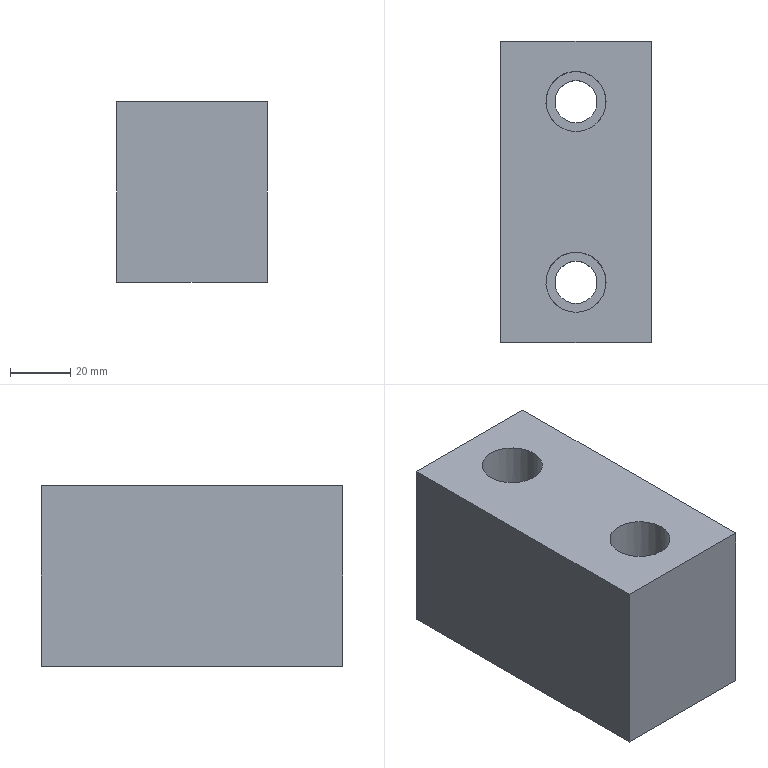Part | NX | features solid 2 | 1 solid | 12 faces | box 50 x 100 x 60 mm | volume 268710 mm3 | plane 8 | cylinder 4 | commonest cylinder face diameters 14 x2 20 x2
STEP:
#1=CARTESIAN_POINT('',(-745.,-395.,-65.));
#2=VERTEX_POINT('',#1);
#3=CARTESIAN_POINT('',(-745.,-295.,-65.));
#4=VERTEX_POINT('',#3);
#5=CARTESIAN_POINT('',(-745.,-400.,-65.));
#6=DIRECTION('',(0.,1.,0.));
#7=VECTOR('',#6,1000.);
#8=LINE('',#5,#7);
#9=EDGE_CURVE('',#2,#4,#8,.T.);
#10=ORIENTED_EDGE('',*,*,#9,.F.);
#11=CARTESIAN_POINT('',(-745.,-395.,-5.));
#12=VERTEX_POINT('',#11);
#13=CARTESIAN_POINT('',(-745.,-395.,-15.));
#14=DIRECTION('',(0.,0.,-1.));
#15=VECTOR('',#14,1000.);
#16=LINE('',#13,#15);
#17=EDGE_CURVE('',#12,#2,#16,.T.);
#18=ORIENTED_EDGE('',*,*,#17,.F.);
#19=CARTESIAN_POINT('',(-745.,-295.,-5.));
#20=VERTEX_POINT('',#19);
#21=CARTESIAN_POINT('',(-745.,-400.,-5.));
#22=DIRECTION('',(0.,-1.,0.));
#23=VECTOR('',#22,1000.);
#24=LINE('',#21,#23);
#25=EDGE_CURVE('',#12,#20,#24,.F.);
#26=ORIENTED_EDGE('',*,*,#25,.T.);
#27=CARTESIAN_POINT('',(-745.,-295.,-15.));
#28=DIRECTION('',(0.,0.,-1.));
#29=VECTOR('',#28,1000.);
#30=LINE('',#27,#29);
#31=EDGE_CURVE('',#20,#4,#30,.T.);
#32=ORIENTED_EDGE('',*,*,#31,.T.);
#33=EDGE_LOOP('',(#10,#18,#26,#32));
#34=FACE_BOUND('',#33,.T.);
#35=CARTESIAN_POINT('',(-745.,-400.,-15.));
#36=DIRECTION('',(1.,0.,0.));
#37=DIRECTION('',(0.,0.,1.));
#38=AXIS2_PLACEMENT_3D('',#35,#36,#37);
#39=PLANE('',#38);
#40=ADVANCED_FACE('',(#34),#39,.F.);
#41=CARTESIAN_POINT('',(-695.,-295.,-65.));
#42=VERTEX_POINT('',#41);
#43=CARTESIAN_POINT('',(-690.,-295.,-65.));
#44=DIRECTION('',(-1.,0.,0.));
#45=VECTOR('',#44,1000.);
#46=LINE('',#43,#45);
#47=EDGE_CURVE('',#42,#4,#46,.T.);
#48=ORIENTED_EDGE('',*,*,#47,.T.);
#49=ORIENTED_EDGE('',*,*,#31,.F.);
#50=CARTESIAN_POINT('',(-695.,-295.,-5.));
#51=VERTEX_POINT('',#50);
#52=CARTESIAN_POINT('',(-690.,-295.,-5.));
#53=DIRECTION('',(1.,0.,0.));
#54=VECTOR('',#53,1000.);
#55=LINE('',#52,#54);
#56=EDGE_CURVE('',#51,#20,#55,.F.);
#57=ORIENTED_EDGE('',*,*,#56,.F.);
#58=CARTESIAN_POINT('',(-695.,-295.,-15.));
#59=DIRECTION('',(0.,0.,-1.));
#60=VECTOR('',#59,1000.);
#61=LINE('',#58,#60);
#62=EDGE_CURVE('',#51,#42,#61,.T.);
#63=ORIENTED_EDGE('',*,*,#62,.T.);
#64=EDGE_LOOP('',(#48,#49,#57,#63));
#65=FACE_BOUND('',#64,.T.);
#66=CARTESIAN_POINT('',(-690.,-295.,-15.));
#67=DIRECTION('',(0.,1.,0.));
#68=DIRECTION('',(0.,0.,-1.));
#69=AXIS2_PLACEMENT_3D('',#66,#67,#68);
#70=PLANE('',#69);
#71=ADVANCED_FACE('',(#65),#70,.T.);
#72=CARTESIAN_POINT('',(-695.,-395.,-65.));
#73=VERTEX_POINT('',#72);
#74=CARTESIAN_POINT('',(-695.,-400.,-65.));
#75=DIRECTION('',(0.,1.,0.));
#76=VECTOR('',#75,1000.);
#77=LINE('',#74,#76);
#78=EDGE_CURVE('',#73,#42,#77,.T.);
#79=ORIENTED_EDGE('',*,*,#78,.T.);
#80=ORIENTED_EDGE('',*,*,#62,.F.);
#81=CARTESIAN_POINT('',(-695.,-395.,-5.));
#82=VERTEX_POINT('',#81);
#83=CARTESIAN_POINT('',(-695.,-400.,-5.));
#84=DIRECTION('',(0.,-1.,0.));
#85=VECTOR('',#84,1000.);
#86=LINE('',#83,#85);
#87=EDGE_CURVE('',#82,#51,#86,.F.);
#88=ORIENTED_EDGE('',*,*,#87,.F.);
#89=CARTESIAN_POINT('',(-695.,-395.,-15.));
#90=DIRECTION('',(0.,0.,-1.));
#91=VECTOR('',#90,1000.);
#92=LINE('',#89,#91);
#93=EDGE_CURVE('',#82,#73,#92,.T.);
#94=ORIENTED_EDGE('',*,*,#93,.T.);
#95=EDGE_LOOP('',(#79,#80,#88,#94));
#96=FACE_BOUND('',#95,.T.);
#97=CARTESIAN_POINT('',(-695.,-400.,-15.));
#98=DIRECTION('',(1.,0.,0.));
#99=DIRECTION('',(0.,0.,1.));
#100=AXIS2_PLACEMENT_3D('',#97,#98,#99);
#101=PLANE('',#100);
#102=ADVANCED_FACE('',(#96),#101,.T.);
#103=CARTESIAN_POINT('',(-690.,-395.,-65.));
#104=DIRECTION('',(-1.,0.,0.));
#105=VECTOR('',#104,1000.);
#106=LINE('',#103,#105);
#107=EDGE_CURVE('',#73,#2,#106,.T.);
#108=ORIENTED_EDGE('',*,*,#107,.F.);
#109=ORIENTED_EDGE('',*,*,#93,.F.);
#110=CARTESIAN_POINT('',(-690.,-395.,-5.));
#111=DIRECTION('',(1.,0.,0.));
#112=VECTOR('',#111,1000.);
#113=LINE('',#110,#112);
#114=EDGE_CURVE('',#82,#12,#113,.F.);
#115=ORIENTED_EDGE('',*,*,#114,.T.);
#116=ORIENTED_EDGE('',*,*,#17,.T.);
#117=EDGE_LOOP('',(#108,#109,#115,#116));
#118=FACE_BOUND('',#117,.T.);
#119=CARTESIAN_POINT('',(-690.,-395.,-15.));
#120=DIRECTION('',(0.,1.,0.));
#121=DIRECTION('',(0.,0.,-1.));
#122=AXIS2_PLACEMENT_3D('',#119,#120,#121);
#123=PLANE('',#122);
#124=ADVANCED_FACE('',(#118),#123,.F.);
#125=CARTESIAN_POINT('',(-710.,-315.,-5.));
#126=VERTEX_POINT('',#125);
#127=CARTESIAN_POINT('',(-720.,-315.,-5.));
#128=DIRECTION('',(0.,0.,1.));
#129=DIRECTION('',(1.,0.,0.));
#130=AXIS2_PLACEMENT_3D('',#127,#128,#129);
#131=CIRCLE('',#130,10.);
#132=EDGE_CURVE('',#126,#126,#131,.T.);
#133=ORIENTED_EDGE('',*,*,#132,.F.);
#134=EDGE_LOOP('',(#133));
#135=FACE_BOUND('',#134,.T.);
#136=CARTESIAN_POINT('',(-710.,-375.,-5.));
#137=VERTEX_POINT('',#136);
#138=CARTESIAN_POINT('',(-720.,-375.,-5.));
#139=DIRECTION('',(0.,0.,1.));
#140=DIRECTION('',(1.,0.,0.));
#141=AXIS2_PLACEMENT_3D('',#138,#139,#140);
#142=CIRCLE('',#141,10.);
#143=EDGE_CURVE('',#137,#137,#142,.T.);
#144=ORIENTED_EDGE('',*,*,#143,.F.);
#145=EDGE_LOOP('',(#144));
#146=FACE_BOUND('',#145,.T.);
#147=ORIENTED_EDGE('',*,*,#25,.F.);
#148=ORIENTED_EDGE('',*,*,#114,.F.);
#149=ORIENTED_EDGE('',*,*,#87,.T.);
#150=ORIENTED_EDGE('',*,*,#56,.T.);
#151=EDGE_LOOP('',(#147,#148,#149,#150));
#152=FACE_BOUND('',#151,.T.);
#153=CARTESIAN_POINT('',(-745.,-295.,-5.));
#154=DIRECTION('',(0.,0.,1.));
#155=DIRECTION('',(1.,0.,0.));
#156=AXIS2_PLACEMENT_3D('',#153,#154,#155);
#157=PLANE('',#156);
#158=ADVANCED_FACE('',(#135,#146,#152),#157,.T.);
#159=CARTESIAN_POINT('',(-720.,-322.,-65.));
#160=VERTEX_POINT('',#159);
#161=CARTESIAN_POINT('',(-720.,-315.,-65.));
#162=DIRECTION('',(0.,0.,-1.));
#163=DIRECTION('',(0.,-1.,0.));
#164=AXIS2_PLACEMENT_3D('',#161,#162,#163);
#165=CIRCLE('',#164,7.);
#166=EDGE_CURVE('',#160,#160,#165,.F.);
#167=ORIENTED_EDGE('',*,*,#166,.T.);
#168=EDGE_LOOP('',(#167));
#169=FACE_BOUND('',#168,.T.);
#170=CARTESIAN_POINT('',(-720.,-382.,-65.));
#171=VERTEX_POINT('',#170);
#172=CARTESIAN_POINT('',(-720.,-375.,-65.));
#173=DIRECTION('',(0.,0.,-1.));
#174=DIRECTION('',(0.,-1.,0.));
#175=AXIS2_PLACEMENT_3D('',#172,#173,#174);
#176=CIRCLE('',#175,7.);
#177=EDGE_CURVE('',#171,#171,#176,.F.);
#178=ORIENTED_EDGE('',*,*,#177,.T.);
#179=EDGE_LOOP('',(#178));
#180=FACE_BOUND('',#179,.T.);
#181=ORIENTED_EDGE('',*,*,#9,.T.);
#182=ORIENTED_EDGE('',*,*,#47,.F.);
#183=ORIENTED_EDGE('',*,*,#78,.F.);
#184=ORIENTED_EDGE('',*,*,#107,.T.);
#185=EDGE_LOOP('',(#181,#182,#183,#184));
#186=FACE_BOUND('',#185,.T.);
#187=CARTESIAN_POINT('',(-690.,-400.,-65.));
#188=DIRECTION('',(0.,0.,-1.));
#189=DIRECTION('',(-1.,0.,0.));
#190=AXIS2_PLACEMENT_3D('',#187,#188,#189);
#191=PLANE('',#190);
#192=ADVANCED_FACE('',(#169,#180,#186),#191,.T.);
#193=CARTESIAN_POINT('',(-720.,-382.,-45.));
#194=VERTEX_POINT('',#193);
#195=CARTESIAN_POINT('',(-720.,-375.,-45.));
#196=DIRECTION('',(0.,0.,-1.));
#197=DIRECTION('',(0.,-1.,0.));
#198=AXIS2_PLACEMENT_3D('',#195,#196,#197);
#199=CIRCLE('',#198,7.);
#200=EDGE_CURVE('',#194,#194,#199,.F.);
#201=ORIENTED_EDGE('',*,*,#200,.F.);
#202=EDGE_LOOP('',(#201));
#203=FACE_BOUND('',#202,.T.);
#204=CARTESIAN_POINT('',(-720.,-385.,-45.));
#205=VERTEX_POINT('',#204);
#206=CARTESIAN_POINT('',(-720.,-375.,-45.));
#207=DIRECTION('',(0.,0.,-1.));
#208=DIRECTION('',(0.,-1.,0.));
#209=AXIS2_PLACEMENT_3D('',#206,#207,#208);
#210=CIRCLE('',#209,10.);
#211=EDGE_CURVE('',#205,#205,#210,.F.);
#212=ORIENTED_EDGE('',*,*,#211,.T.);
#213=EDGE_LOOP('',(#212));
#214=FACE_BOUND('',#213,.T.);
#215=CARTESIAN_POINT('',(-720.,-375.,-45.));
#216=DIRECTION('',(0.,0.,-1.));
#217=DIRECTION('',(0.,-1.,0.));
#218=AXIS2_PLACEMENT_3D('',#215,#216,#217);
#219=PLANE('',#218);
#220=ADVANCED_FACE('',(#203,#214),#219,.F.);
#221=ORIENTED_EDGE('',*,*,#211,.F.);
#222=EDGE_LOOP('',(#221));
#223=FACE_BOUND('',#222,.T.);
#224=ORIENTED_EDGE('',*,*,#143,.T.);
#225=EDGE_LOOP('',(#224));
#226=FACE_BOUND('',#225,.T.);
#227=CARTESIAN_POINT('',(-720.,-375.,-15.));
#228=DIRECTION('',(0.,0.,-1.));
#229=DIRECTION('',(0.,-1.,0.));
#230=AXIS2_PLACEMENT_3D('',#227,#228,#229);
#231=CYLINDRICAL_SURFACE('',#230,10.);
#232=ADVANCED_FACE('',(#223,#226),#231,.F.);
#233=CARTESIAN_POINT('',(-720.,-322.,-45.));
#234=VERTEX_POINT('',#233);
#235=CARTESIAN_POINT('',(-720.,-315.,-45.));
#236=DIRECTION('',(0.,0.,-1.));
#237=DIRECTION('',(0.,-1.,0.));
#238=AXIS2_PLACEMENT_3D('',#235,#236,#237);
#239=CIRCLE('',#238,7.);
#240=EDGE_CURVE('',#234,#234,#239,.F.);
#241=ORIENTED_EDGE('',*,*,#240,.F.);
#242=EDGE_LOOP('',(#241));
#243=FACE_BOUND('',#242,.T.);
#244=CARTESIAN_POINT('',(-720.,-325.,-45.));
#245=VERTEX_POINT('',#244);
#246=CARTESIAN_POINT('',(-720.,-315.,-45.));
#247=DIRECTION('',(0.,0.,-1.));
#248=DIRECTION('',(0.,-1.,0.));
#249=AXIS2_PLACEMENT_3D('',#246,#247,#248);
#250=CIRCLE('',#249,10.);
#251=EDGE_CURVE('',#245,#245,#250,.F.);
#252=ORIENTED_EDGE('',*,*,#251,.T.);
#253=EDGE_LOOP('',(#252));
#254=FACE_BOUND('',#253,.T.);
#255=CARTESIAN_POINT('',(-720.,-315.,-45.));
#256=DIRECTION('',(0.,0.,-1.));
#257=DIRECTION('',(0.,-1.,0.));
#258=AXIS2_PLACEMENT_3D('',#255,#256,#257);
#259=PLANE('',#258);
#260=ADVANCED_FACE('',(#243,#254),#259,.F.);
#261=ORIENTED_EDGE('',*,*,#251,.F.);
#262=EDGE_LOOP('',(#261));
#263=FACE_BOUND('',#262,.T.);
#264=ORIENTED_EDGE('',*,*,#132,.T.);
#265=EDGE_LOOP('',(#264));
#266=FACE_BOUND('',#265,.T.);
#267=CARTESIAN_POINT('',(-720.,-315.,-15.));
#268=DIRECTION('',(0.,0.,-1.));
#269=DIRECTION('',(0.,-1.,0.));
#270=AXIS2_PLACEMENT_3D('',#267,#268,#269);
#271=CYLINDRICAL_SURFACE('',#270,10.);
#272=ADVANCED_FACE('',(#263,#266),#271,.F.);
#273=ORIENTED_EDGE('',*,*,#177,.F.);
#274=EDGE_LOOP('',(#273));
#275=FACE_BOUND('',#274,.T.);
#276=ORIENTED_EDGE('',*,*,#200,.T.);
#277=EDGE_LOOP('',(#276));
#278=FACE_BOUND('',#277,.T.);
#279=CARTESIAN_POINT('',(-720.,-375.,-45.));
#280=DIRECTION('',(0.,0.,-1.));
#281=DIRECTION('',(0.,-1.,0.));
#282=AXIS2_PLACEMENT_3D('',#279,#280,#281);
#283=CYLINDRICAL_SURFACE('',#282,7.);
#284=ADVANCED_FACE('',(#275,#278),#283,.F.);
#285=ORIENTED_EDGE('',*,*,#166,.F.);
#286=EDGE_LOOP('',(#285));
#287=FACE_BOUND('',#286,.T.);
#288=ORIENTED_EDGE('',*,*,#240,.T.);
#289=EDGE_LOOP('',(#288));
#290=FACE_BOUND('',#289,.T.);
#291=CARTESIAN_POINT('',(-720.,-315.,-45.));
#292=DIRECTION('',(0.,0.,-1.));
#293=DIRECTION('',(0.,-1.,0.));
#294=AXIS2_PLACEMENT_3D('',#291,#292,#293);
#295=CYLINDRICAL_SURFACE('',#294,7.);
#296=ADVANCED_FACE('',(#287,#290),#295,.F.);
#297=CLOSED_SHELL('',(#40,#71,#102,#124,#158,#192,#220,#232,#260,#272,#284,#296));
#298=MANIFOLD_SOLID_BREP('',#297);
#299=(LENGTH_UNIT()NAMED_UNIT(*)SI_UNIT(.MILLI.,.METRE.));
#300=UNCERTAINTY_MEASURE_WITH_UNIT(LENGTH_MEASURE(0.00001),#299,'','');
#301=(NAMED_UNIT(*)PLANE_ANGLE_UNIT()SI_UNIT($,.RADIAN.));
#302=(NAMED_UNIT(*)SI_UNIT($,.STERADIAN.)SOLID_ANGLE_UNIT());
#303=(GEOMETRIC_REPRESENTATION_CONTEXT(3)GLOBAL_UNCERTAINTY_ASSIGNED_CONTEXT((#300))GLOBAL_UNIT_ASSIGNED_CONTEXT((#299,#301,#302))REPRESENTATION_CONTEXT('',''));
#304=ADVANCED_BREP_SHAPE_REPRESENTATION('',(#298),#303);